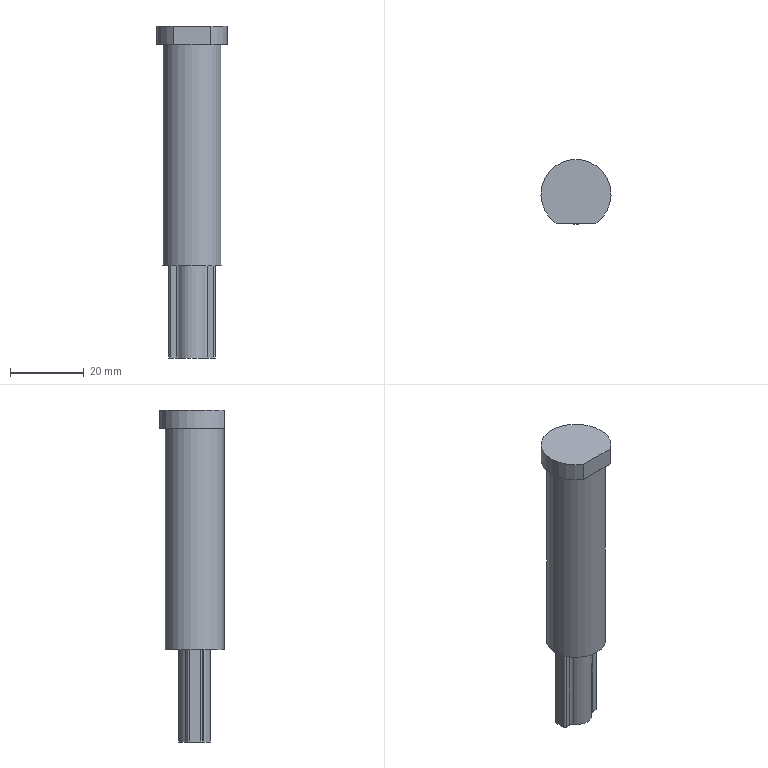Part | NX | features solid 2 | 1 solid | 23 faces | box 19 x 17.5 x 90 mm | volume 15280 mm3 | cylinder 12 | plane 11 | commonest cylinder face diameters 1 x4 2 x4 8.5 x2 16 x1 19 x1
STEP:
#1=CARTESIAN_POINT('',(43.829,-293.974,14.));
#2=VERTEX_POINT('',#1);
#3=CARTESIAN_POINT('',(43.829,-301.974,14.));
#4=DIRECTION('',(0.,0.,1.));
#5=DIRECTION('',(0.,1.,0.));
#6=AXIS2_PLACEMENT_3D('',#3,#4,#5);
#7=CIRCLE('',#6,8.);
#8=EDGE_CURVE('',#2,#2,#7,.T.);
#9=ORIENTED_EDGE('',*,*,#8,.F.);
#10=EDGE_LOOP('',(#9));
#11=FACE_BOUND('',#10,.T.);
#12=CARTESIAN_POINT('',(48.138,-303.974,14.));
#13=VERTEX_POINT('',#12);
#14=CARTESIAN_POINT('',(47.317,-304.402,14.));
#15=VERTEX_POINT('',#14);
#16=CARTESIAN_POINT('',(48.138,-304.974,14.));
#17=DIRECTION('',(0.,0.,1.));
#18=DIRECTION('',(-1.,0.,0.));
#19=AXIS2_PLACEMENT_3D('',#16,#17,#18);
#20=CIRCLE('',#19,1.);
#21=EDGE_CURVE('',#13,#15,#20,.T.);
#22=ORIENTED_EDGE('',*,*,#21,.F.);
#23=CARTESIAN_POINT('',(49.579,-303.974,14.));
#24=VERTEX_POINT('',#23);
#25=CARTESIAN_POINT('',(43.829,-303.974,14.));
#26=DIRECTION('',(-1.,0.,0.));
#27=VECTOR('',#26,1000.);
#28=LINE('',#25,#27);
#29=EDGE_CURVE('',#24,#13,#28,.T.);
#30=ORIENTED_EDGE('',*,*,#29,.F.);
#31=CARTESIAN_POINT('',(50.079,-303.474,14.));
#32=VERTEX_POINT('',#31);
#33=CARTESIAN_POINT('',(49.579,-303.474,14.));
#34=DIRECTION('',(0.,0.,1.));
#35=DIRECTION('',(-1.,0.,0.));
#36=AXIS2_PLACEMENT_3D('',#33,#34,#35);
#37=CIRCLE('',#36,0.5);
#38=EDGE_CURVE('',#24,#32,#37,.T.);
#39=ORIENTED_EDGE('',*,*,#38,.T.);
#40=CARTESIAN_POINT('',(50.079,-300.474,14.));
#41=VERTEX_POINT('',#40);
#42=CARTESIAN_POINT('',(50.079,-301.974,14.));
#43=DIRECTION('',(-0.000003944,1.,0.));
#44=VECTOR('',#43,1000.);
#45=LINE('',#42,#44);
#46=EDGE_CURVE('',#32,#41,#45,.T.);
#47=ORIENTED_EDGE('',*,*,#46,.T.);
#48=CARTESIAN_POINT('',(49.579,-299.974,14.));
#49=VERTEX_POINT('',#48);
#50=CARTESIAN_POINT('',(49.579,-300.474,14.));
#51=DIRECTION('',(0.,0.,1.));
#52=DIRECTION('',(-1.,0.,0.));
#53=AXIS2_PLACEMENT_3D('',#50,#51,#52);
#54=CIRCLE('',#53,0.5);
#55=EDGE_CURVE('',#41,#49,#54,.T.);
#56=ORIENTED_EDGE('',*,*,#55,.T.);
#57=CARTESIAN_POINT('',(48.138,-299.974,14.));
#58=VERTEX_POINT('',#57);
#59=CARTESIAN_POINT('',(43.829,-299.974,14.));
#60=DIRECTION('',(-1.,0.,0.));
#61=VECTOR('',#60,1000.);
#62=LINE('',#59,#61);
#63=EDGE_CURVE('',#49,#58,#62,.T.);
#64=ORIENTED_EDGE('',*,*,#63,.T.);
#65=CARTESIAN_POINT('',(47.317,-299.545,14.));
#66=VERTEX_POINT('',#65);
#67=CARTESIAN_POINT('',(48.138,-298.974,14.));
#68=DIRECTION('',(0.,0.,1.));
#69=DIRECTION('',(-1.,0.,0.));
#70=AXIS2_PLACEMENT_3D('',#67,#68,#69);
#71=CIRCLE('',#70,1.);
#72=EDGE_CURVE('',#66,#58,#71,.T.);
#73=ORIENTED_EDGE('',*,*,#72,.F.);
#74=CARTESIAN_POINT('',(40.342,-299.545,14.));
#75=VERTEX_POINT('',#74);
#76=CARTESIAN_POINT('',(43.829,-301.974,14.));
#77=DIRECTION('',(0.,0.,1.));
#78=DIRECTION('',(-1.,0.,0.));
#79=AXIS2_PLACEMENT_3D('',#76,#77,#78);
#80=CIRCLE('',#79,4.25);
#81=EDGE_CURVE('',#66,#75,#80,.T.);
#82=ORIENTED_EDGE('',*,*,#81,.T.);
#83=CARTESIAN_POINT('',(39.521,-299.974,14.));
#84=VERTEX_POINT('',#83);
#85=CARTESIAN_POINT('',(39.521,-298.974,14.));
#86=DIRECTION('',(0.,0.,1.));
#87=DIRECTION('',(-1.,0.,0.));
#88=AXIS2_PLACEMENT_3D('',#85,#86,#87);
#89=CIRCLE('',#88,1.);
#90=EDGE_CURVE('',#84,#75,#89,.T.);
#91=ORIENTED_EDGE('',*,*,#90,.F.);
#92=CARTESIAN_POINT('',(38.079,-299.974,14.));
#93=VERTEX_POINT('',#92);
#94=CARTESIAN_POINT('',(43.829,-299.974,14.));
#95=DIRECTION('',(-1.,0.,0.));
#96=VECTOR('',#95,1000.);
#97=LINE('',#94,#96);
#98=EDGE_CURVE('',#84,#93,#97,.T.);
#99=ORIENTED_EDGE('',*,*,#98,.T.);
#100=CARTESIAN_POINT('',(37.579,-300.474,14.));
#101=VERTEX_POINT('',#100);
#102=CARTESIAN_POINT('',(38.079,-300.474,14.));
#103=DIRECTION('',(0.,0.,1.));
#104=DIRECTION('',(-1.,0.,0.));
#105=AXIS2_PLACEMENT_3D('',#102,#103,#104);
#106=CIRCLE('',#105,0.5);
#107=EDGE_CURVE('',#93,#101,#106,.T.);
#108=ORIENTED_EDGE('',*,*,#107,.T.);
#109=CARTESIAN_POINT('',(37.579,-303.474,14.));
#110=VERTEX_POINT('',#109);
#111=CARTESIAN_POINT('',(37.579,-301.974,14.));
#112=DIRECTION('',(-0.000003944,1.,0.));
#113=VECTOR('',#112,1000.);
#114=LINE('',#111,#113);
#115=EDGE_CURVE('',#110,#101,#114,.T.);
#116=ORIENTED_EDGE('',*,*,#115,.F.);
#117=CARTESIAN_POINT('',(38.079,-303.974,14.));
#118=VERTEX_POINT('',#117);
#119=CARTESIAN_POINT('',(38.079,-303.474,14.));
#120=DIRECTION('',(0.,0.,1.));
#121=DIRECTION('',(-1.,0.,0.));
#122=AXIS2_PLACEMENT_3D('',#119,#120,#121);
#123=CIRCLE('',#122,0.5);
#124=EDGE_CURVE('',#110,#118,#123,.T.);
#125=ORIENTED_EDGE('',*,*,#124,.T.);
#126=CARTESIAN_POINT('',(39.521,-303.974,14.));
#127=VERTEX_POINT('',#126);
#128=CARTESIAN_POINT('',(43.829,-303.974,14.));
#129=DIRECTION('',(-1.,0.,0.));
#130=VECTOR('',#129,1000.);
#131=LINE('',#128,#130);
#132=EDGE_CURVE('',#127,#118,#131,.T.);
#133=ORIENTED_EDGE('',*,*,#132,.F.);
#134=CARTESIAN_POINT('',(40.342,-304.402,14.));
#135=VERTEX_POINT('',#134);
#136=CARTESIAN_POINT('',(39.521,-304.974,14.));
#137=DIRECTION('',(0.,0.,1.));
#138=DIRECTION('',(-1.,0.,0.));
#139=AXIS2_PLACEMENT_3D('',#136,#137,#138);
#140=CIRCLE('',#139,1.);
#141=EDGE_CURVE('',#135,#127,#140,.T.);
#142=ORIENTED_EDGE('',*,*,#141,.F.);
#143=CARTESIAN_POINT('',(43.829,-301.974,14.));
#144=DIRECTION('',(0.,0.,1.));
#145=DIRECTION('',(-1.,0.,0.));
#146=AXIS2_PLACEMENT_3D('',#143,#144,#145);
#147=CIRCLE('',#146,4.25);
#148=EDGE_CURVE('',#135,#15,#147,.T.);
#149=ORIENTED_EDGE('',*,*,#148,.T.);
#150=EDGE_LOOP('',(#22,#30,#39,#47,#56,#64,#73,#82,#91,#99,#108,#116,#125,#133,#142,#149));
#151=FACE_BOUND('',#150,.T.);
#152=CARTESIAN_POINT('',(43.829,-301.974,14.));
#153=DIRECTION('',(0.,0.,1.));
#154=DIRECTION('',(0.,1.,0.));
#155=AXIS2_PLACEMENT_3D('',#152,#153,#154);
#156=PLANE('',#155);
#157=ADVANCED_FACE('',(#11,#151),#156,.F.);
#158=ORIENTED_EDGE('',*,*,#8,.T.);
#159=EDGE_LOOP('',(#158));
#160=FACE_BOUND('',#159,.T.);
#161=CARTESIAN_POINT('',(43.829,-309.974,74.));
#162=VERTEX_POINT('',#161);
#163=CARTESIAN_POINT('',(43.829,-301.974,74.));
#164=DIRECTION('',(0.,0.,1.));
#165=DIRECTION('',(0.,1.,0.));
#166=AXIS2_PLACEMENT_3D('',#163,#164,#165);
#167=CIRCLE('',#166,8.);
#168=EDGE_CURVE('',#162,#162,#167,.T.);
#169=ORIENTED_EDGE('',*,*,#168,.F.);
#170=EDGE_LOOP('',(#169));
#171=FACE_BOUND('',#170,.T.);
#172=CARTESIAN_POINT('',(43.829,-301.974,79.));
#173=DIRECTION('',(0.,0.,-1.));
#174=DIRECTION('',(0.,-1.,0.));
#175=AXIS2_PLACEMENT_3D('',#172,#173,#174);
#176=CYLINDRICAL_SURFACE('',#175,8.);
#177=ADVANCED_FACE('',(#160,#171),#176,.T.);
#178=CARTESIAN_POINT('',(48.953,-309.974,74.));
#179=VERTEX_POINT('',#178);
#180=CARTESIAN_POINT('',(38.706,-309.974,74.));
#181=VERTEX_POINT('',#180);
#182=CARTESIAN_POINT('',(43.829,-301.974,74.));
#183=DIRECTION('',(0.,0.,1.));
#184=DIRECTION('',(0.,1.,0.));
#185=AXIS2_PLACEMENT_3D('',#182,#183,#184);
#186=CIRCLE('',#185,9.5);
#187=EDGE_CURVE('',#179,#181,#186,.T.);
#188=ORIENTED_EDGE('',*,*,#187,.F.);
#189=CARTESIAN_POINT('',(43.829,-309.974,74.));
#190=DIRECTION('',(-1.,0.,0.));
#191=VECTOR('',#190,1000.);
#192=LINE('',#189,#191);
#193=EDGE_CURVE('',#179,#162,#192,.T.);
#194=ORIENTED_EDGE('',*,*,#193,.T.);
#195=ORIENTED_EDGE('',*,*,#168,.T.);
#196=CARTESIAN_POINT('',(43.829,-309.974,74.));
#197=DIRECTION('',(-1.,0.,0.));
#198=VECTOR('',#197,1000.);
#199=LINE('',#196,#198);
#200=EDGE_CURVE('',#162,#181,#199,.T.);
#201=ORIENTED_EDGE('',*,*,#200,.T.);
#202=EDGE_LOOP('',(#188,#194,#195,#201));
#203=FACE_BOUND('',#202,.T.);
#204=CARTESIAN_POINT('',(43.829,-301.974,74.));
#205=DIRECTION('',(0.,0.,1.));
#206=DIRECTION('',(0.,1.,0.));
#207=AXIS2_PLACEMENT_3D('',#204,#205,#206);
#208=PLANE('',#207);
#209=ADVANCED_FACE('',(#203),#208,.F.);
#210=CARTESIAN_POINT('',(38.706,-309.974,79.));
#211=VERTEX_POINT('',#210);
#212=CARTESIAN_POINT('',(38.706,-309.974,83.));
#213=DIRECTION('',(0.,0.,-1.));
#214=VECTOR('',#213,1000.);
#215=LINE('',#212,#214);
#216=EDGE_CURVE('',#211,#181,#215,.T.);
#217=ORIENTED_EDGE('',*,*,#216,.F.);
#218=CARTESIAN_POINT('',(48.953,-309.974,79.));
#219=VERTEX_POINT('',#218);
#220=CARTESIAN_POINT('',(43.829,-301.974,79.));
#221=DIRECTION('',(0.,0.,1.));
#222=DIRECTION('',(0.,1.,0.));
#223=AXIS2_PLACEMENT_3D('',#220,#221,#222);
#224=CIRCLE('',#223,9.5);
#225=EDGE_CURVE('',#219,#211,#224,.T.);
#226=ORIENTED_EDGE('',*,*,#225,.F.);
#227=CARTESIAN_POINT('',(48.953,-309.974,83.));
#228=DIRECTION('',(0.,0.,-1.));
#229=VECTOR('',#228,1000.);
#230=LINE('',#227,#229);
#231=EDGE_CURVE('',#179,#219,#230,.F.);
#232=ORIENTED_EDGE('',*,*,#231,.F.);
#233=ORIENTED_EDGE('',*,*,#187,.T.);
#234=EDGE_LOOP('',(#217,#226,#232,#233));
#235=FACE_BOUND('',#234,.T.);
#236=CARTESIAN_POINT('',(43.829,-301.974,74.));
#237=DIRECTION('',(0.,0.,1.));
#238=DIRECTION('',(0.,1.,0.));
#239=AXIS2_PLACEMENT_3D('',#236,#237,#238);
#240=CYLINDRICAL_SURFACE('',#239,9.5);
#241=ADVANCED_FACE('',(#235),#240,.T.);
#242=CARTESIAN_POINT('',(43.829,-309.974,79.));
#243=DIRECTION('',(-1.,0.,0.));
#244=VECTOR('',#243,1000.);
#245=LINE('',#242,#244);
#246=EDGE_CURVE('',#219,#211,#245,.T.);
#247=ORIENTED_EDGE('',*,*,#246,.F.);
#248=ORIENTED_EDGE('',*,*,#225,.T.);
#249=EDGE_LOOP('',(#247,#248));
#250=FACE_BOUND('',#249,.T.);
#251=CARTESIAN_POINT('',(43.829,-301.974,79.));
#252=DIRECTION('',(0.,0.,1.));
#253=DIRECTION('',(0.,1.,0.));
#254=AXIS2_PLACEMENT_3D('',#251,#252,#253);
#255=PLANE('',#254);
#256=ADVANCED_FACE('',(#250),#255,.T.);
#257=ORIENTED_EDGE('',*,*,#231,.T.);
#258=ORIENTED_EDGE('',*,*,#246,.T.);
#259=ORIENTED_EDGE('',*,*,#216,.T.);
#260=ORIENTED_EDGE('',*,*,#200,.F.);
#261=ORIENTED_EDGE('',*,*,#193,.F.);
#262=EDGE_LOOP('',(#257,#258,#259,#260,#261));
#263=FACE_BOUND('',#262,.T.);
#264=CARTESIAN_POINT('',(38.706,-309.974,83.));
#265=DIRECTION('',(0.,1.,0.));
#266=DIRECTION('',(-1.,0.,0.));
#267=AXIS2_PLACEMENT_3D('',#264,#265,#266);
#268=PLANE('',#267);
#269=ADVANCED_FACE('',(#263),#268,.F.);
#270=CARTESIAN_POINT('',(48.138,-303.974,-11.));
#271=VERTEX_POINT('',#270);
#272=CARTESIAN_POINT('',(48.138,-303.974,-57.));
#273=DIRECTION('',(0.,0.,1.));
#274=VECTOR('',#273,1000.);
#275=LINE('',#272,#274);
#276=EDGE_CURVE('',#271,#13,#275,.T.);
#277=ORIENTED_EDGE('',*,*,#276,.T.);
#278=ORIENTED_EDGE('',*,*,#21,.T.);
#279=CARTESIAN_POINT('',(47.317,-304.402,-11.));
#280=VERTEX_POINT('',#279);
#281=CARTESIAN_POINT('',(47.317,-304.402,-57.));
#282=DIRECTION('',(0.,0.,1.));
#283=VECTOR('',#282,1000.);
#284=LINE('',#281,#283);
#285=EDGE_CURVE('',#280,#15,#284,.T.);
#286=ORIENTED_EDGE('',*,*,#285,.F.);
#287=CARTESIAN_POINT('',(48.138,-304.974,-11.));
#288=DIRECTION('',(0.,0.,1.));
#289=DIRECTION('',(-1.,0.,0.));
#290=AXIS2_PLACEMENT_3D('',#287,#288,#289);
#291=CIRCLE('',#290,1.);
#292=EDGE_CURVE('',#271,#280,#291,.T.);
#293=ORIENTED_EDGE('',*,*,#292,.F.);
#294=EDGE_LOOP('',(#277,#278,#286,#293));
#295=FACE_BOUND('',#294,.T.);
#296=CARTESIAN_POINT('',(48.138,-304.974,-57.));
#297=DIRECTION('',(0.,0.,1.));
#298=DIRECTION('',(-1.,0.,0.));
#299=AXIS2_PLACEMENT_3D('',#296,#297,#298);
#300=CYLINDRICAL_SURFACE('',#299,1.);
#301=ADVANCED_FACE('',(#295),#300,.F.);
#302=ORIENTED_EDGE('',*,*,#148,.F.);
#303=CARTESIAN_POINT('',(40.342,-304.402,-11.));
#304=VERTEX_POINT('',#303);
#305=CARTESIAN_POINT('',(40.342,-304.402,-57.));
#306=DIRECTION('',(0.,0.,1.));
#307=VECTOR('',#306,1000.);
#308=LINE('',#305,#307);
#309=EDGE_CURVE('',#304,#135,#308,.T.);
#310=ORIENTED_EDGE('',*,*,#309,.F.);
#311=CARTESIAN_POINT('',(43.829,-301.974,-11.));
#312=DIRECTION('',(0.,0.,1.));
#313=DIRECTION('',(-1.,0.,0.));
#314=AXIS2_PLACEMENT_3D('',#311,#312,#313);
#315=CIRCLE('',#314,4.25);
#316=EDGE_CURVE('',#304,#280,#315,.T.);
#317=ORIENTED_EDGE('',*,*,#316,.T.);
#318=ORIENTED_EDGE('',*,*,#285,.T.);
#319=EDGE_LOOP('',(#302,#310,#317,#318));
#320=FACE_BOUND('',#319,.T.);
#321=CARTESIAN_POINT('',(43.829,-301.974,-57.));
#322=DIRECTION('',(0.,0.,1.));
#323=DIRECTION('',(-1.,0.,0.));
#324=AXIS2_PLACEMENT_3D('',#321,#322,#323);
#325=CYLINDRICAL_SURFACE('',#324,4.25);
#326=ADVANCED_FACE('',(#320),#325,.T.);
#327=ORIENTED_EDGE('',*,*,#309,.T.);
#328=ORIENTED_EDGE('',*,*,#141,.T.);
#329=CARTESIAN_POINT('',(39.521,-303.974,-11.));
#330=VERTEX_POINT('',#329);
#331=CARTESIAN_POINT('',(39.521,-303.974,-57.));
#332=DIRECTION('',(0.,0.,1.));
#333=VECTOR('',#332,1000.);
#334=LINE('',#331,#333);
#335=EDGE_CURVE('',#330,#127,#334,.T.);
#336=ORIENTED_EDGE('',*,*,#335,.F.);
#337=CARTESIAN_POINT('',(39.521,-304.974,-11.));
#338=DIRECTION('',(0.,0.,1.));
#339=DIRECTION('',(-1.,0.,0.));
#340=AXIS2_PLACEMENT_3D('',#337,#338,#339);
#341=CIRCLE('',#340,1.);
#342=EDGE_CURVE('',#304,#330,#341,.T.);
#343=ORIENTED_EDGE('',*,*,#342,.F.);
#344=EDGE_LOOP('',(#327,#328,#336,#343));
#345=FACE_BOUND('',#344,.T.);
#346=CARTESIAN_POINT('',(39.521,-304.974,-57.));
#347=DIRECTION('',(0.,0.,1.));
#348=DIRECTION('',(-1.,0.,0.));
#349=AXIS2_PLACEMENT_3D('',#346,#347,#348);
#350=CYLINDRICAL_SURFACE('',#349,1.);
#351=ADVANCED_FACE('',(#345),#350,.F.);
#352=ORIENTED_EDGE('',*,*,#335,.T.);
#353=ORIENTED_EDGE('',*,*,#132,.T.);
#354=CARTESIAN_POINT('',(38.079,-303.974,-11.));
#355=VERTEX_POINT('',#354);
#356=CARTESIAN_POINT('',(38.079,-303.974,-57.));
#357=DIRECTION('',(0.,0.,1.));
#358=VECTOR('',#357,1000.);
#359=LINE('',#356,#358);
#360=EDGE_CURVE('',#355,#118,#359,.T.);
#361=ORIENTED_EDGE('',*,*,#360,.F.);
#362=CARTESIAN_POINT('',(45.829,-303.974,-11.));
#363=DIRECTION('',(-1.,0.,0.));
#364=VECTOR('',#363,1000.);
#365=LINE('',#362,#364);
#366=EDGE_CURVE('',#330,#355,#365,.T.);
#367=ORIENTED_EDGE('',*,*,#366,.F.);
#368=EDGE_LOOP('',(#352,#353,#361,#367));
#369=FACE_BOUND('',#368,.T.);
#370=CARTESIAN_POINT('',(39.521,-303.974,-57.));
#371=DIRECTION('',(0.,1.,0.));
#372=DIRECTION('',(0.,0.,-1.));
#373=AXIS2_PLACEMENT_3D('',#370,#371,#372);
#374=PLANE('',#373);
#375=ADVANCED_FACE('',(#369),#374,.F.);
#376=ORIENTED_EDGE('',*,*,#124,.F.);
#377=CARTESIAN_POINT('',(37.579,-303.474,-11.));
#378=VERTEX_POINT('',#377);
#379=CARTESIAN_POINT('',(37.579,-303.474,-57.));
#380=DIRECTION('',(0.,0.,1.));
#381=VECTOR('',#380,1000.);
#382=LINE('',#379,#381);
#383=EDGE_CURVE('',#378,#110,#382,.T.);
#384=ORIENTED_EDGE('',*,*,#383,.F.);
#385=CARTESIAN_POINT('',(38.079,-303.474,-11.));
#386=DIRECTION('',(0.,0.,1.));
#387=DIRECTION('',(-1.,0.,0.));
#388=AXIS2_PLACEMENT_3D('',#385,#386,#387);
#389=CIRCLE('',#388,0.5);
#390=EDGE_CURVE('',#378,#355,#389,.T.);
#391=ORIENTED_EDGE('',*,*,#390,.T.);
#392=ORIENTED_EDGE('',*,*,#360,.T.);
#393=EDGE_LOOP('',(#376,#384,#391,#392));
#394=FACE_BOUND('',#393,.T.);
#395=CARTESIAN_POINT('',(38.079,-303.474,-57.));
#396=DIRECTION('',(0.,0.,1.));
#397=DIRECTION('',(-1.,0.,0.));
#398=AXIS2_PLACEMENT_3D('',#395,#396,#397);
#399=CYLINDRICAL_SURFACE('',#398,0.5);
#400=ADVANCED_FACE('',(#394),#399,.T.);
#401=ORIENTED_EDGE('',*,*,#383,.T.);
#402=ORIENTED_EDGE('',*,*,#115,.T.);
#403=CARTESIAN_POINT('',(37.579,-300.474,-11.));
#404=VERTEX_POINT('',#403);
#405=CARTESIAN_POINT('',(37.579,-300.474,-57.));
#406=DIRECTION('',(0.,0.,1.));
#407=VECTOR('',#406,1000.);
#408=LINE('',#405,#407);
#409=EDGE_CURVE('',#404,#101,#408,.T.);
#410=ORIENTED_EDGE('',*,*,#409,.F.);
#411=CARTESIAN_POINT('',(37.579,-301.974,-11.));
#412=DIRECTION('',(-0.000003944,1.,0.));
#413=VECTOR('',#412,1000.);
#414=LINE('',#411,#413);
#415=EDGE_CURVE('',#378,#404,#414,.T.);
#416=ORIENTED_EDGE('',*,*,#415,.F.);
#417=EDGE_LOOP('',(#401,#402,#410,#416));
#418=FACE_BOUND('',#417,.T.);
#419=CARTESIAN_POINT('',(37.579,-303.474,-57.));
#420=DIRECTION('',(1.,0.000003944,0.));
#421=DIRECTION('',(-0.000003944,1.,0.));
#422=AXIS2_PLACEMENT_3D('',#419,#420,#421);
#423=PLANE('',#422);
#424=ADVANCED_FACE('',(#418),#423,.F.);
#425=ORIENTED_EDGE('',*,*,#107,.F.);
#426=CARTESIAN_POINT('',(38.079,-299.974,-11.));
#427=VERTEX_POINT('',#426);
#428=CARTESIAN_POINT('',(38.079,-299.974,-57.));
#429=DIRECTION('',(0.,0.,1.));
#430=VECTOR('',#429,1000.);
#431=LINE('',#428,#430);
#432=EDGE_CURVE('',#427,#93,#431,.T.);
#433=ORIENTED_EDGE('',*,*,#432,.F.);
#434=CARTESIAN_POINT('',(38.079,-300.474,-11.));
#435=DIRECTION('',(0.,0.,1.));
#436=DIRECTION('',(-1.,0.,0.));
#437=AXIS2_PLACEMENT_3D('',#434,#435,#436);
#438=CIRCLE('',#437,0.5);
#439=EDGE_CURVE('',#427,#404,#438,.T.);
#440=ORIENTED_EDGE('',*,*,#439,.T.);
#441=ORIENTED_EDGE('',*,*,#409,.T.);
#442=EDGE_LOOP('',(#425,#433,#440,#441));
#443=FACE_BOUND('',#442,.T.);
#444=CARTESIAN_POINT('',(38.079,-300.474,-57.));
#445=DIRECTION('',(0.,0.,1.));
#446=DIRECTION('',(-1.,0.,0.));
#447=AXIS2_PLACEMENT_3D('',#444,#445,#446);
#448=CYLINDRICAL_SURFACE('',#447,0.5);
#449=ADVANCED_FACE('',(#443),#448,.T.);
#450=ORIENTED_EDGE('',*,*,#98,.F.);
#451=CARTESIAN_POINT('',(39.521,-299.974,-11.));
#452=VERTEX_POINT('',#451);
#453=CARTESIAN_POINT('',(39.521,-299.974,-57.));
#454=DIRECTION('',(0.,0.,1.));
#455=VECTOR('',#454,1000.);
#456=LINE('',#453,#455);
#457=EDGE_CURVE('',#452,#84,#456,.T.);
#458=ORIENTED_EDGE('',*,*,#457,.F.);
#459=CARTESIAN_POINT('',(45.829,-299.974,-11.));
#460=DIRECTION('',(-1.,0.,0.));
#461=VECTOR('',#460,1000.);
#462=LINE('',#459,#461);
#463=EDGE_CURVE('',#452,#427,#462,.T.);
#464=ORIENTED_EDGE('',*,*,#463,.T.);
#465=ORIENTED_EDGE('',*,*,#432,.T.);
#466=EDGE_LOOP('',(#450,#458,#464,#465));
#467=FACE_BOUND('',#466,.T.);
#468=CARTESIAN_POINT('',(39.521,-299.974,-57.));
#469=DIRECTION('',(0.,1.,0.));
#470=DIRECTION('',(0.,0.,-1.));
#471=AXIS2_PLACEMENT_3D('',#468,#469,#470);
#472=PLANE('',#471);
#473=ADVANCED_FACE('',(#467),#472,.T.);
#474=ORIENTED_EDGE('',*,*,#457,.T.);
#475=ORIENTED_EDGE('',*,*,#90,.T.);
#476=CARTESIAN_POINT('',(40.342,-299.545,-11.));
#477=VERTEX_POINT('',#476);
#478=CARTESIAN_POINT('',(40.342,-299.545,-57.));
#479=DIRECTION('',(0.,0.,1.));
#480=VECTOR('',#479,1000.);
#481=LINE('',#478,#480);
#482=EDGE_CURVE('',#477,#75,#481,.T.);
#483=ORIENTED_EDGE('',*,*,#482,.F.);
#484=CARTESIAN_POINT('',(39.521,-298.974,-11.));
#485=DIRECTION('',(0.,0.,1.));
#486=DIRECTION('',(-1.,0.,0.));
#487=AXIS2_PLACEMENT_3D('',#484,#485,#486);
#488=CIRCLE('',#487,1.);
#489=EDGE_CURVE('',#452,#477,#488,.T.);
#490=ORIENTED_EDGE('',*,*,#489,.F.);
#491=EDGE_LOOP('',(#474,#475,#483,#490));
#492=FACE_BOUND('',#491,.T.);
#493=CARTESIAN_POINT('',(39.521,-298.974,-57.));
#494=DIRECTION('',(0.,0.,1.));
#495=DIRECTION('',(-1.,0.,0.));
#496=AXIS2_PLACEMENT_3D('',#493,#494,#495);
#497=CYLINDRICAL_SURFACE('',#496,1.);
#498=ADVANCED_FACE('',(#492),#497,.F.);
#499=ORIENTED_EDGE('',*,*,#81,.F.);
#500=CARTESIAN_POINT('',(47.317,-299.545,-11.));
#501=VERTEX_POINT('',#500);
#502=CARTESIAN_POINT('',(47.317,-299.545,-57.));
#503=DIRECTION('',(0.,0.,1.));
#504=VECTOR('',#503,1000.);
#505=LINE('',#502,#504);
#506=EDGE_CURVE('',#501,#66,#505,.T.);
#507=ORIENTED_EDGE('',*,*,#506,.F.);
#508=CARTESIAN_POINT('',(43.829,-301.974,-11.));
#509=DIRECTION('',(0.,0.,1.));
#510=DIRECTION('',(-1.,0.,0.));
#511=AXIS2_PLACEMENT_3D('',#508,#509,#510);
#512=CIRCLE('',#511,4.25);
#513=EDGE_CURVE('',#501,#477,#512,.T.);
#514=ORIENTED_EDGE('',*,*,#513,.T.);
#515=ORIENTED_EDGE('',*,*,#482,.T.);
#516=EDGE_LOOP('',(#499,#507,#514,#515));
#517=FACE_BOUND('',#516,.T.);
#518=CARTESIAN_POINT('',(43.829,-301.974,-57.));
#519=DIRECTION('',(0.,0.,1.));
#520=DIRECTION('',(-1.,0.,0.));
#521=AXIS2_PLACEMENT_3D('',#518,#519,#520);
#522=CYLINDRICAL_SURFACE('',#521,4.25);
#523=ADVANCED_FACE('',(#517),#522,.T.);
#524=ORIENTED_EDGE('',*,*,#506,.T.);
#525=ORIENTED_EDGE('',*,*,#72,.T.);
#526=CARTESIAN_POINT('',(48.138,-299.974,-11.));
#527=VERTEX_POINT('',#526);
#528=CARTESIAN_POINT('',(48.138,-299.974,-57.));
#529=DIRECTION('',(0.,0.,1.));
#530=VECTOR('',#529,1000.);
#531=LINE('',#528,#530);
#532=EDGE_CURVE('',#527,#58,#531,.T.);
#533=ORIENTED_EDGE('',*,*,#532,.F.);
#534=CARTESIAN_POINT('',(48.138,-298.974,-11.));
#535=DIRECTION('',(0.,0.,1.));
#536=DIRECTION('',(-1.,0.,0.));
#537=AXIS2_PLACEMENT_3D('',#534,#535,#536);
#538=CIRCLE('',#537,1.);
#539=EDGE_CURVE('',#501,#527,#538,.T.);
#540=ORIENTED_EDGE('',*,*,#539,.F.);
#541=EDGE_LOOP('',(#524,#525,#533,#540));
#542=FACE_BOUND('',#541,.T.);
#543=CARTESIAN_POINT('',(48.138,-298.974,-57.));
#544=DIRECTION('',(0.,0.,1.));
#545=DIRECTION('',(-1.,0.,0.));
#546=AXIS2_PLACEMENT_3D('',#543,#544,#545);
#547=CYLINDRICAL_SURFACE('',#546,1.);
#548=ADVANCED_FACE('',(#542),#547,.F.);
#549=ORIENTED_EDGE('',*,*,#63,.F.);
#550=CARTESIAN_POINT('',(49.579,-299.974,-11.));
#551=VERTEX_POINT('',#550);
#552=CARTESIAN_POINT('',(49.579,-299.974,-57.));
#553=DIRECTION('',(0.,0.,1.));
#554=VECTOR('',#553,1000.);
#555=LINE('',#552,#554);
#556=EDGE_CURVE('',#551,#49,#555,.T.);
#557=ORIENTED_EDGE('',*,*,#556,.F.);
#558=CARTESIAN_POINT('',(45.829,-299.974,-11.));
#559=DIRECTION('',(-1.,0.,0.));
#560=VECTOR('',#559,1000.);
#561=LINE('',#558,#560);
#562=EDGE_CURVE('',#551,#527,#561,.T.);
#563=ORIENTED_EDGE('',*,*,#562,.T.);
#564=ORIENTED_EDGE('',*,*,#532,.T.);
#565=EDGE_LOOP('',(#549,#557,#563,#564));
#566=FACE_BOUND('',#565,.T.);
#567=CARTESIAN_POINT('',(49.579,-299.974,-57.));
#568=DIRECTION('',(0.,1.,0.));
#569=DIRECTION('',(0.,0.,-1.));
#570=AXIS2_PLACEMENT_3D('',#567,#568,#569);
#571=PLANE('',#570);
#572=ADVANCED_FACE('',(#566),#571,.T.);
#573=ORIENTED_EDGE('',*,*,#55,.F.);
#574=CARTESIAN_POINT('',(50.079,-300.474,-11.));
#575=VERTEX_POINT('',#574);
#576=CARTESIAN_POINT('',(50.079,-300.474,-57.));
#577=DIRECTION('',(0.,0.,1.));
#578=VECTOR('',#577,1000.);
#579=LINE('',#576,#578);
#580=EDGE_CURVE('',#575,#41,#579,.T.);
#581=ORIENTED_EDGE('',*,*,#580,.F.);
#582=CARTESIAN_POINT('',(49.579,-300.474,-11.));
#583=DIRECTION('',(0.,0.,1.));
#584=DIRECTION('',(-1.,0.,0.));
#585=AXIS2_PLACEMENT_3D('',#582,#583,#584);
#586=CIRCLE('',#585,0.5);
#587=EDGE_CURVE('',#575,#551,#586,.T.);
#588=ORIENTED_EDGE('',*,*,#587,.T.);
#589=ORIENTED_EDGE('',*,*,#556,.T.);
#590=EDGE_LOOP('',(#573,#581,#588,#589));
#591=FACE_BOUND('',#590,.T.);
#592=CARTESIAN_POINT('',(49.579,-300.474,-57.));
#593=DIRECTION('',(0.,0.,1.));
#594=DIRECTION('',(-1.,0.,0.));
#595=AXIS2_PLACEMENT_3D('',#592,#593,#594);
#596=CYLINDRICAL_SURFACE('',#595,0.5);
#597=ADVANCED_FACE('',(#591),#596,.T.);
#598=ORIENTED_EDGE('',*,*,#46,.F.);
#599=CARTESIAN_POINT('',(50.079,-303.474,-11.));
#600=VERTEX_POINT('',#599);
#601=CARTESIAN_POINT('',(50.079,-303.474,-57.));
#602=DIRECTION('',(0.,0.,1.));
#603=VECTOR('',#602,1000.);
#604=LINE('',#601,#603);
#605=EDGE_CURVE('',#600,#32,#604,.T.);
#606=ORIENTED_EDGE('',*,*,#605,.F.);
#607=CARTESIAN_POINT('',(50.079,-301.974,-11.));
#608=DIRECTION('',(-0.000003944,1.,0.));
#609=VECTOR('',#608,1000.);
#610=LINE('',#607,#609);
#611=EDGE_CURVE('',#600,#575,#610,.T.);
#612=ORIENTED_EDGE('',*,*,#611,.T.);
#613=ORIENTED_EDGE('',*,*,#580,.T.);
#614=EDGE_LOOP('',(#598,#606,#612,#613));
#615=FACE_BOUND('',#614,.T.);
#616=CARTESIAN_POINT('',(50.079,-303.474,-57.));
#617=DIRECTION('',(1.,0.000003944,0.));
#618=DIRECTION('',(-0.000003944,1.,0.));
#619=AXIS2_PLACEMENT_3D('',#616,#617,#618);
#620=PLANE('',#619);
#621=ADVANCED_FACE('',(#615),#620,.T.);
#622=ORIENTED_EDGE('',*,*,#38,.F.);
#623=CARTESIAN_POINT('',(49.579,-303.974,-11.));
#624=VERTEX_POINT('',#623);
#625=CARTESIAN_POINT('',(49.579,-303.974,-57.));
#626=DIRECTION('',(0.,0.,1.));
#627=VECTOR('',#626,1000.);
#628=LINE('',#625,#627);
#629=EDGE_CURVE('',#624,#24,#628,.T.);
#630=ORIENTED_EDGE('',*,*,#629,.F.);
#631=CARTESIAN_POINT('',(49.579,-303.474,-11.));
#632=DIRECTION('',(0.,0.,1.));
#633=DIRECTION('',(-1.,0.,0.));
#634=AXIS2_PLACEMENT_3D('',#631,#632,#633);
#635=CIRCLE('',#634,0.5);
#636=EDGE_CURVE('',#624,#600,#635,.T.);
#637=ORIENTED_EDGE('',*,*,#636,.T.);
#638=ORIENTED_EDGE('',*,*,#605,.T.);
#639=EDGE_LOOP('',(#622,#630,#637,#638));
#640=FACE_BOUND('',#639,.T.);
#641=CARTESIAN_POINT('',(49.579,-303.474,-57.));
#642=DIRECTION('',(0.,0.,1.));
#643=DIRECTION('',(-1.,0.,0.));
#644=AXIS2_PLACEMENT_3D('',#641,#642,#643);
#645=CYLINDRICAL_SURFACE('',#644,0.5);
#646=ADVANCED_FACE('',(#640),#645,.T.);
#647=ORIENTED_EDGE('',*,*,#629,.T.);
#648=ORIENTED_EDGE('',*,*,#29,.T.);
#649=ORIENTED_EDGE('',*,*,#276,.F.);
#650=CARTESIAN_POINT('',(45.829,-303.974,-11.));
#651=DIRECTION('',(-1.,0.,0.));
#652=VECTOR('',#651,1000.);
#653=LINE('',#650,#652);
#654=EDGE_CURVE('',#624,#271,#653,.T.);
#655=ORIENTED_EDGE('',*,*,#654,.F.);
#656=EDGE_LOOP('',(#647,#648,#649,#655));
#657=FACE_BOUND('',#656,.T.);
#658=CARTESIAN_POINT('',(49.579,-303.974,-57.));
#659=DIRECTION('',(0.,1.,0.));
#660=DIRECTION('',(0.,0.,-1.));
#661=AXIS2_PLACEMENT_3D('',#658,#659,#660);
#662=PLANE('',#661);
#663=ADVANCED_FACE('',(#657),#662,.F.);
#664=ORIENTED_EDGE('',*,*,#292,.T.);
#665=ORIENTED_EDGE('',*,*,#316,.F.);
#666=ORIENTED_EDGE('',*,*,#342,.T.);
#667=ORIENTED_EDGE('',*,*,#366,.T.);
#668=ORIENTED_EDGE('',*,*,#390,.F.);
#669=ORIENTED_EDGE('',*,*,#415,.T.);
#670=ORIENTED_EDGE('',*,*,#439,.F.);
#671=ORIENTED_EDGE('',*,*,#463,.F.);
#672=ORIENTED_EDGE('',*,*,#489,.T.);
#673=ORIENTED_EDGE('',*,*,#513,.F.);
#674=ORIENTED_EDGE('',*,*,#539,.T.);
#675=ORIENTED_EDGE('',*,*,#562,.F.);
#676=ORIENTED_EDGE('',*,*,#587,.F.);
#677=ORIENTED_EDGE('',*,*,#611,.F.);
#678=ORIENTED_EDGE('',*,*,#636,.F.);
#679=ORIENTED_EDGE('',*,*,#654,.T.);
#680=EDGE_LOOP('',(#664,#665,#666,#667,#668,#669,#670,#671,#672,#673,#674,#675,#676,#677,#678,#679));
#681=FACE_BOUND('',#680,.T.);
#682=CARTESIAN_POINT('',(45.829,-301.974,-11.));
#683=DIRECTION('',(0.,0.,1.));
#684=DIRECTION('',(0.,1.,0.));
#685=AXIS2_PLACEMENT_3D('',#682,#683,#684);
#686=PLANE('',#685);
#687=ADVANCED_FACE('',(#681),#686,.F.);
#688=CLOSED_SHELL('',(#157,#177,#209,#241,#256,#269,#301,#326,#351,#375,#400,#424,#449,#473,#498,#523,#548,#572,#597,#621,#646,#663,#687));
#689=MANIFOLD_SOLID_BREP('',#688);
#690=(LENGTH_UNIT()NAMED_UNIT(*)SI_UNIT(.MILLI.,.METRE.));
#691=UNCERTAINTY_MEASURE_WITH_UNIT(LENGTH_MEASURE(0.00001),#690,'','');
#692=(NAMED_UNIT(*)PLANE_ANGLE_UNIT()SI_UNIT($,.RADIAN.));
#693=(NAMED_UNIT(*)SI_UNIT($,.STERADIAN.)SOLID_ANGLE_UNIT());
#694=(GEOMETRIC_REPRESENTATION_CONTEXT(3)GLOBAL_UNCERTAINTY_ASSIGNED_CONTEXT((#691))GLOBAL_UNIT_ASSIGNED_CONTEXT((#690,#692,#693))REPRESENTATION_CONTEXT('',''));
#695=ADVANCED_BREP_SHAPE_REPRESENTATION('',(#689),#694);